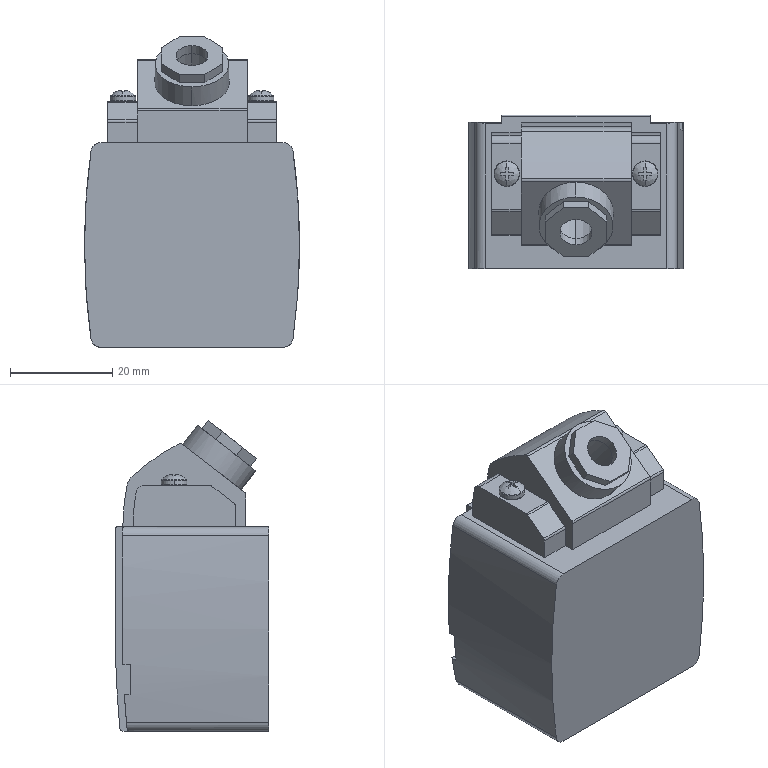Part | SolidWorks | features BaseBody 1 | 1 solid | 137 faces | box 42.009 x 30.001 x 60.7 mm | volume 55286 mm3 | plane 76 | cylinder 49 | spline 12 | commonest cylinder face diameters 1.2 x12 2.8 x8 4 x6 5 x4 400 x4 3 x2